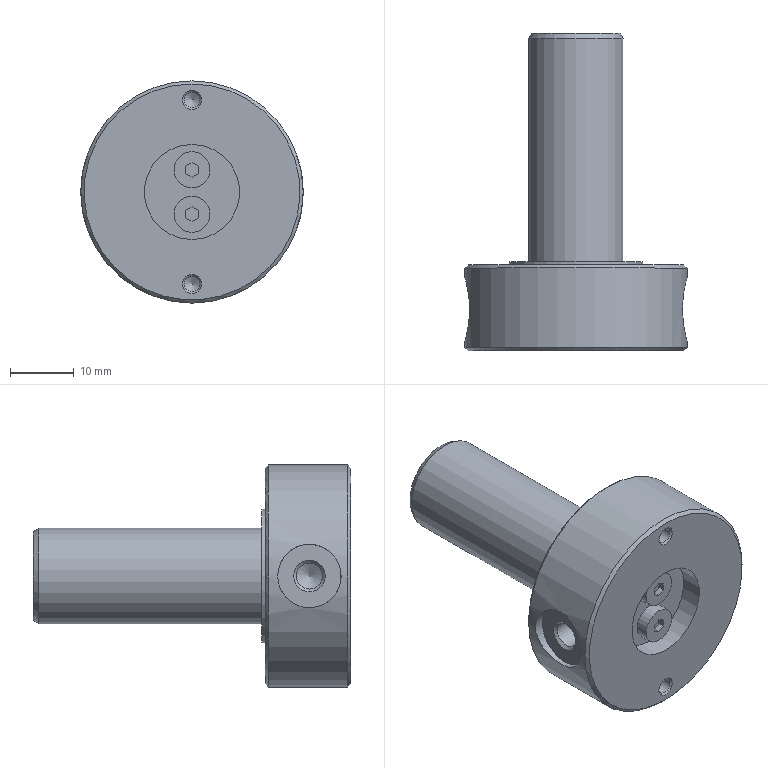Part | NX | 1 solid | 51 faces | box 35 x 50 x 35 mm | volume 18431 mm3 | plane 24 | cylinder 14 | cone 13 | commonest cylinder face diameters 2.459 x2 4.134 x2 5.7 x2 10 x2 15 x2 3 x1
STEP:
#1=CARTESIAN_POINT('',(0.,14.,-7.5));
#2=VERTEX_POINT('',#1);
#3=CARTESIAN_POINT('',(0.,14.,0.));
#4=DIRECTION('',(0.,-1.,0.));
#5=DIRECTION('',(0.,0.,-1.));
#6=AXIS2_PLACEMENT_3D('',#3,#4,#5);
#7=CIRCLE('',#6,7.5);
#8=EDGE_CURVE('',#2,#2,#7,.F.);
#9=ORIENTED_EDGE('',*,*,#8,.T.);
#10=EDGE_LOOP('',(#9));
#11=FACE_BOUND('',#10,.T.);
#12=CARTESIAN_POINT('',(0.,49.13,-7.5));
#13=VERTEX_POINT('',#12);
#14=CARTESIAN_POINT('',(0.,49.13,0.));
#15=DIRECTION('',(0.,-1.,0.));
#16=DIRECTION('',(0.,0.,-1.));
#17=AXIS2_PLACEMENT_3D('',#14,#15,#16);
#18=CIRCLE('',#17,7.5);
#19=EDGE_CURVE('',#13,#13,#18,.T.);
#20=ORIENTED_EDGE('',*,*,#19,.T.);
#21=EDGE_LOOP('',(#20));
#22=FACE_BOUND('',#21,.T.);
#23=CARTESIAN_POINT('',(0.,31.565,0.));
#24=DIRECTION('',(0.,-1.,0.));
#25=DIRECTION('',(0.,0.,-1.));
#26=AXIS2_PLACEMENT_3D('',#23,#24,#25);
#27=CYLINDRICAL_SURFACE('',#26,7.5);
#28=ADVANCED_FACE('',(#11,#22),#27,.T.);
#29=CARTESIAN_POINT('',(0.,50.,-7.));
#30=VERTEX_POINT('',#29);
#31=CARTESIAN_POINT('',(0.,50.,0.));
#32=DIRECTION('',(0.,-1.,0.));
#33=DIRECTION('',(0.,0.,-1.));
#34=AXIS2_PLACEMENT_3D('',#31,#32,#33);
#35=CIRCLE('',#34,7.);
#36=EDGE_CURVE('',#30,#30,#35,.T.);
#37=ORIENTED_EDGE('',*,*,#36,.T.);
#38=EDGE_LOOP('',(#37));
#39=FACE_BOUND('',#38,.T.);
#40=ORIENTED_EDGE('',*,*,#19,.F.);
#41=EDGE_LOOP('',(#40));
#42=FACE_BOUND('',#41,.T.);
#43=CARTESIAN_POINT('',(0.,49.13,0.));
#44=DIRECTION('',(0.,-1.,0.));
#45=DIRECTION('',(0.,0.,-1.));
#46=AXIS2_PLACEMENT_3D('',#43,#44,#45);
#47=CONICAL_SURFACE('',#46,7.5,0.5216);
#48=ADVANCED_FACE('',(#39,#42),#47,.T.);
#49=CARTESIAN_POINT('',(0.,14.,-10.5));
#50=VERTEX_POINT('',#49);
#51=CARTESIAN_POINT('',(0.,14.,0.));
#52=DIRECTION('',(0.,-1.,0.));
#53=DIRECTION('',(0.,0.,-1.));
#54=AXIS2_PLACEMENT_3D('',#51,#52,#53);
#55=CIRCLE('',#54,10.5);
#56=EDGE_CURVE('',#50,#50,#55,.F.);
#57=ORIENTED_EDGE('',*,*,#56,.T.);
#58=EDGE_LOOP('',(#57));
#59=FACE_BOUND('',#58,.T.);
#60=ORIENTED_EDGE('',*,*,#8,.F.);
#61=EDGE_LOOP('',(#60));
#62=FACE_BOUND('',#61,.T.);
#63=CARTESIAN_POINT('',(9.,14.,0.));
#64=DIRECTION('',(0.,1.,0.));
#65=DIRECTION('',(0.,0.,1.));
#66=AXIS2_PLACEMENT_3D('',#63,#64,#65);
#67=PLANE('',#66);
#68=ADVANCED_FACE('',(#59,#62),#67,.T.);
#69=ORIENTED_EDGE('',*,*,#36,.F.);
#70=EDGE_LOOP('',(#69));
#71=FACE_BOUND('',#70,.T.);
#72=CARTESIAN_POINT('',(0.,50.,2.));
#73=VERTEX_POINT('',#72);
#74=CARTESIAN_POINT('',(0.,50.,0.));
#75=DIRECTION('',(0.,1.,0.));
#76=DIRECTION('',(0.,0.,1.));
#77=AXIS2_PLACEMENT_3D('',#74,#75,#76);
#78=CIRCLE('',#77,2.);
#79=EDGE_CURVE('',#73,#73,#78,.F.);
#80=ORIENTED_EDGE('',*,*,#79,.T.);
#81=EDGE_LOOP('',(#80));
#82=FACE_BOUND('',#81,.T.);
#83=CARTESIAN_POINT('',(0.,50.,-6.));
#84=VERTEX_POINT('',#83);
#85=CARTESIAN_POINT('',(0.,50.,-4.5));
#86=DIRECTION('',(0.,-1.,0.));
#87=DIRECTION('',(0.,0.,-1.));
#88=AXIS2_PLACEMENT_3D('',#85,#86,#87);
#89=CIRCLE('',#88,1.5);
#90=EDGE_CURVE('',#84,#84,#89,.T.);
#91=ORIENTED_EDGE('',*,*,#90,.T.);
#92=EDGE_LOOP('',(#91));
#93=FACE_BOUND('',#92,.T.);
#94=CARTESIAN_POINT('',(3.5,50.,0.));
#95=DIRECTION('',(0.,1.,0.));
#96=DIRECTION('',(0.,0.,1.));
#97=AXIS2_PLACEMENT_3D('',#94,#95,#96);
#98=PLANE('',#97);
#99=ADVANCED_FACE('',(#71,#82,#93),#98,.T.);
#100=ORIENTED_EDGE('',*,*,#56,.F.);
#101=EDGE_LOOP('',(#100));
#102=FACE_BOUND('',#101,.T.);
#103=CARTESIAN_POINT('',(0.,13.5,-10.5));
#104=VERTEX_POINT('',#103);
#105=CARTESIAN_POINT('',(0.,13.5,0.));
#106=DIRECTION('',(0.,-1.,0.));
#107=DIRECTION('',(0.,0.,-1.));
#108=AXIS2_PLACEMENT_3D('',#105,#106,#107);
#109=CIRCLE('',#108,10.5);
#110=EDGE_CURVE('',#104,#104,#109,.F.);
#111=ORIENTED_EDGE('',*,*,#110,.T.);
#112=EDGE_LOOP('',(#111));
#113=FACE_BOUND('',#112,.T.);
#114=CARTESIAN_POINT('',(0.,13.75,0.));
#115=DIRECTION('',(0.,-1.,0.));
#116=DIRECTION('',(0.,0.,-1.));
#117=AXIS2_PLACEMENT_3D('',#114,#115,#116);
#118=CYLINDRICAL_SURFACE('',#117,10.5);
#119=ADVANCED_FACE('',(#102,#113),#118,.T.);
#120=ORIENTED_EDGE('',*,*,#79,.F.);
#121=EDGE_LOOP('',(#120));
#122=FACE_BOUND('',#121,.T.);
#123=CARTESIAN_POINT('',(1.621,49.621,0.));
#124=VERTEX_POINT('',#123);
#125=CARTESIAN_POINT('',(0.,49.621,0.));
#126=DIRECTION('',(0.,1.,0.));
#127=DIRECTION('',(1.,0.,0.));
#128=AXIS2_PLACEMENT_3D('',#125,#126,#127);
#129=CIRCLE('',#128,1.621);
#130=EDGE_CURVE('',#124,#124,#129,.T.);
#131=ORIENTED_EDGE('',*,*,#130,.F.);
#132=EDGE_LOOP('',(#131));
#133=FACE_BOUND('',#132,.T.);
#134=CARTESIAN_POINT('',(0.,50.,0.));
#135=DIRECTION('',(0.,1.,0.));
#136=DIRECTION('',(0.,0.,1.));
#137=AXIS2_PLACEMENT_3D('',#134,#135,#136);
#138=CONICAL_SURFACE('',#137,2.,0.7854);
#139=ADVANCED_FACE('',(#122,#133),#138,.F.);
#140=ORIENTED_EDGE('',*,*,#90,.F.);
#141=EDGE_LOOP('',(#140));
#142=FACE_BOUND('',#141,.T.);
#143=CARTESIAN_POINT('',(0.,40.,-6.));
#144=VERTEX_POINT('',#143);
#145=CARTESIAN_POINT('',(0.,40.,-4.5));
#146=DIRECTION('',(0.,-1.,0.));
#147=DIRECTION('',(0.,0.,-1.));
#148=AXIS2_PLACEMENT_3D('',#145,#146,#147);
#149=CIRCLE('',#148,1.5);
#150=EDGE_CURVE('',#144,#144,#149,.F.);
#151=ORIENTED_EDGE('',*,*,#150,.F.);
#152=EDGE_LOOP('',(#151));
#153=FACE_BOUND('',#152,.T.);
#154=CARTESIAN_POINT('',(0.,45.,-4.5));
#155=DIRECTION('',(0.,-1.,0.));
#156=DIRECTION('',(0.,0.,-1.));
#157=AXIS2_PLACEMENT_3D('',#154,#155,#156);
#158=CYLINDRICAL_SURFACE('',#157,1.5);
#159=ADVANCED_FACE('',(#142,#153),#158,.F.);
#160=CARTESIAN_POINT('',(0.,13.5,-17.));
#161=VERTEX_POINT('',#160);
#162=CARTESIAN_POINT('',(0.,13.5,0.));
#163=DIRECTION('',(0.,-1.,0.));
#164=DIRECTION('',(0.,0.,-1.));
#165=AXIS2_PLACEMENT_3D('',#162,#163,#164);
#166=CIRCLE('',#165,17.);
#167=EDGE_CURVE('',#161,#161,#166,.F.);
#168=ORIENTED_EDGE('',*,*,#167,.T.);
#169=EDGE_LOOP('',(#168));
#170=FACE_BOUND('',#169,.T.);
#171=ORIENTED_EDGE('',*,*,#110,.F.);
#172=EDGE_LOOP('',(#171));
#173=FACE_BOUND('',#172,.T.);
#174=CARTESIAN_POINT('',(13.75,13.5,0.));
#175=DIRECTION('',(0.,1.,0.));
#176=DIRECTION('',(0.,0.,1.));
#177=AXIS2_PLACEMENT_3D('',#174,#175,#176);
#178=PLANE('',#177);
#179=ADVANCED_FACE('',(#170,#173),#178,.T.);
#180=ORIENTED_EDGE('',*,*,#130,.T.);
#181=EDGE_LOOP('',(#180));
#182=FACE_BOUND('',#181,.T.);
#183=CARTESIAN_POINT('',(0.,42.,-1.621));
#184=VERTEX_POINT('',#183);
#185=CARTESIAN_POINT('',(0.,42.,0.));
#186=DIRECTION('',(0.,-1.,0.));
#187=DIRECTION('',(0.,0.,-1.));
#188=AXIS2_PLACEMENT_3D('',#185,#186,#187);
#189=CIRCLE('',#188,1.621);
#190=EDGE_CURVE('',#184,#184,#189,.F.);
#191=ORIENTED_EDGE('',*,*,#190,.F.);
#192=EDGE_LOOP('',(#191));
#193=FACE_BOUND('',#192,.T.);
#194=CARTESIAN_POINT('',(0.,45.81,0.));
#195=DIRECTION('',(0.,-1.,0.));
#196=DIRECTION('',(0.,0.,-1.));
#197=AXIS2_PLACEMENT_3D('',#194,#195,#196);
#198=CYLINDRICAL_SURFACE('',#197,1.621);
#199=ADVANCED_FACE('',(#182,#193),#198,.F.);
#200=ORIENTED_EDGE('',*,*,#150,.T.);
#201=EDGE_LOOP('',(#200));
#202=FACE_BOUND('',#201,.T.);
#203=CARTESIAN_POINT('',(0.,40.,-5.25));
#204=DIRECTION('',(0.,-1.,0.));
#205=DIRECTION('',(0.,0.,-1.));
#206=AXIS2_PLACEMENT_3D('',#203,#204,#205);
#207=PLANE('',#206);
#208=ADVANCED_FACE('',(#202),#207,.F.);
#209=ORIENTED_EDGE('',*,*,#167,.F.);
#210=EDGE_LOOP('',(#209));
#211=FACE_BOUND('',#210,.T.);
#212=CARTESIAN_POINT('',(17.5,13.,0.));
#213=VERTEX_POINT('',#212);
#214=CARTESIAN_POINT('',(0.,13.,0.));
#215=DIRECTION('',(0.,-1.,0.));
#216=DIRECTION('',(1.,0.,0.));
#217=AXIS2_PLACEMENT_3D('',#214,#215,#216);
#218=CIRCLE('',#217,17.5);
#219=EDGE_CURVE('',#213,#213,#218,.F.);
#220=ORIENTED_EDGE('',*,*,#219,.T.);
#221=EDGE_LOOP('',(#220));
#222=FACE_BOUND('',#221,.T.);
#223=CARTESIAN_POINT('',(0.,13.,0.));
#224=DIRECTION('',(0.,-1.,0.));
#225=DIRECTION('',(0.,0.,-1.));
#226=AXIS2_PLACEMENT_3D('',#223,#224,#225);
#227=CONICAL_SURFACE('',#226,17.5,0.7854);
#228=ADVANCED_FACE('',(#211,#222),#227,.T.);
#229=CARTESIAN_POINT('',(0.,41.064,0.));
#230=VERTEX_POINT('',#229);
#231=VERTEX_LOOP('',#230);
#232=FACE_BOUND('',#231,.T.);
#233=ORIENTED_EDGE('',*,*,#190,.T.);
#234=EDGE_LOOP('',(#233));
#235=FACE_BOUND('',#234,.T.);
#236=CARTESIAN_POINT('',(0.,42.,0.));
#237=DIRECTION('',(0.,1.,0.));
#238=DIRECTION('',(0.,0.,1.));
#239=AXIS2_PLACEMENT_3D('',#236,#237,#238);
#240=CONICAL_SURFACE('',#239,1.621,1.047);
#241=ADVANCED_FACE('',(#232,#235),#240,.F.);
#242=CARTESIAN_POINT('',(17.5,1.5,0.));
#243=VERTEX_POINT('',#242);
#244=CARTESIAN_POINT('',(17.143,2.584,-3.92));
#245=CARTESIAN_POINT('',(17.679,0.9588,0.0006164));
#246=CARTESIAN_POINT('',(17.143,2.581,3.917));
#247=CARTESIAN_POINT('',(16.584,6.501,5.541));
#248=CARTESIAN_POINT('',(17.143,10.416,3.92));
#249=CARTESIAN_POINT('',(17.679,12.041,-0.00121));
#250=CARTESIAN_POINT('',(17.143,10.419,-3.917));
#251=CARTESIAN_POINT('',(16.584,6.499,-5.541));
#252=CARTESIAN_POINT('',(17.143,2.584,-3.92));
#253=CARTESIAN_POINT('',(17.679,0.9588,0.0006164));
#254=CARTESIAN_POINT('',(17.143,2.581,3.917));
#255=B_SPLINE_CURVE_WITH_KNOTS('',3,(#244,#245,#246,#247,#248,#249,#250,#251,#252,#253,#254),.UNSPECIFIED.,.T.,.F.,(1,1,1,1,1,1,1,1,1,1,1,1,1,1,1),(-0.01963,-0.0157,-0.01178,-0.007852,-0.003926,0.000000332,0.003926,0.007852,0.01178,0.0157,0.01963,0.02356,0.02748,0.03141,0.03533),.UNSPECIFIED.);
#256=EDGE_CURVE('',#243,#243,#255,.T.);
#257=ORIENTED_EDGE('',*,*,#256,.T.);
#258=EDGE_LOOP('',(#257));
#259=FACE_BOUND('',#258,.T.);
#260=ORIENTED_EDGE('',*,*,#219,.F.);
#261=EDGE_LOOP('',(#260));
#262=FACE_BOUND('',#261,.T.);
#263=CARTESIAN_POINT('',(-17.5,11.5,0.));
#264=VERTEX_POINT('',#263);
#265=CARTESIAN_POINT('',(-17.143,10.416,-3.92));
#266=CARTESIAN_POINT('',(-17.679,12.041,0.0006164));
#267=CARTESIAN_POINT('',(-17.143,10.419,3.917));
#268=CARTESIAN_POINT('',(-16.584,6.499,5.541));
#269=CARTESIAN_POINT('',(-17.143,2.584,3.92));
#270=CARTESIAN_POINT('',(-17.679,0.9588,-0.00121));
#271=CARTESIAN_POINT('',(-17.143,2.581,-3.917));
#272=CARTESIAN_POINT('',(-16.584,6.501,-5.541));
#273=CARTESIAN_POINT('',(-17.143,10.416,-3.92));
#274=CARTESIAN_POINT('',(-17.679,12.041,0.0006164));
#275=CARTESIAN_POINT('',(-17.143,10.419,3.917));
#276=B_SPLINE_CURVE_WITH_KNOTS('',3,(#265,#266,#267,#268,#269,#270,#271,#272,#273,#274,#275),.UNSPECIFIED.,.T.,.F.,(1,1,1,1,1,1,1,1,1,1,1,1,1,1,1),(-0.01963,-0.0157,-0.01178,-0.007852,-0.003926,0.000000332,0.003926,0.007852,0.01178,0.0157,0.01963,0.02356,0.02748,0.03141,0.03533),.UNSPECIFIED.);
#277=EDGE_CURVE('',#264,#264,#276,.T.);
#278=ORIENTED_EDGE('',*,*,#277,.T.);
#279=EDGE_LOOP('',(#278));
#280=FACE_BOUND('',#279,.T.);
#281=CARTESIAN_POINT('',(0.,0.5,-17.5));
#282=VERTEX_POINT('',#281);
#283=CARTESIAN_POINT('',(0.,0.5,0.));
#284=DIRECTION('',(0.,-1.,0.));
#285=DIRECTION('',(0.,0.,-1.));
#286=AXIS2_PLACEMENT_3D('',#283,#284,#285);
#287=CIRCLE('',#286,17.5);
#288=EDGE_CURVE('',#282,#282,#287,.F.);
#289=ORIENTED_EDGE('',*,*,#288,.T.);
#290=EDGE_LOOP('',(#289));
#291=FACE_BOUND('',#290,.T.);
#292=CARTESIAN_POINT('',(0.,6.75,0.));
#293=DIRECTION('',(0.,-1.,0.));
#294=DIRECTION('',(0.,0.,-1.));
#295=AXIS2_PLACEMENT_3D('',#292,#293,#294);
#296=CYLINDRICAL_SURFACE('',#295,17.5);
#297=ADVANCED_FACE('',(#259,#262,#280,#291),#296,.T.);
#298=ORIENTED_EDGE('',*,*,#288,.F.);
#299=EDGE_LOOP('',(#298));
#300=FACE_BOUND('',#299,.T.);
#301=CARTESIAN_POINT('',(0.,0.,17.));
#302=VERTEX_POINT('',#301);
#303=CARTESIAN_POINT('',(0.,0.,0.));
#304=DIRECTION('',(0.,1.,0.));
#305=DIRECTION('',(0.,0.,1.));
#306=AXIS2_PLACEMENT_3D('',#303,#304,#305);
#307=CIRCLE('',#306,17.);
#308=EDGE_CURVE('',#302,#302,#307,.T.);
#309=ORIENTED_EDGE('',*,*,#308,.T.);
#310=EDGE_LOOP('',(#309));
#311=FACE_BOUND('',#310,.T.);
#312=CARTESIAN_POINT('',(0.,0.5,0.));
#313=DIRECTION('',(0.,1.,0.));
#314=DIRECTION('',(0.,0.,1.));
#315=AXIS2_PLACEMENT_3D('',#312,#313,#314);
#316=CONICAL_SURFACE('',#315,17.5,0.7854);
#317=ADVANCED_FACE('',(#300,#311),#316,.T.);
#318=CARTESIAN_POINT('',(-16.,6.5,5.));
#319=VERTEX_POINT('',#318);
#320=CARTESIAN_POINT('',(-16.,6.5,0.));
#321=DIRECTION('',(-1.,0.,0.));
#322=DIRECTION('',(0.,0.,1.));
#323=AXIS2_PLACEMENT_3D('',#320,#321,#322);
#324=CIRCLE('',#323,5.);
#325=EDGE_CURVE('',#319,#319,#324,.T.);
#326=ORIENTED_EDGE('',*,*,#325,.F.);
#327=EDGE_LOOP('',(#326));
#328=FACE_BOUND('',#327,.T.);
#329=ORIENTED_EDGE('',*,*,#277,.F.);
#330=EDGE_LOOP('',(#329));
#331=FACE_BOUND('',#330,.T.);
#332=CARTESIAN_POINT('',(-16.75,6.5,0.));
#333=DIRECTION('',(-1.,0.,0.));
#334=DIRECTION('',(0.,0.,1.));
#335=AXIS2_PLACEMENT_3D('',#332,#333,#334);
#336=CYLINDRICAL_SURFACE('',#335,5.);
#337=ADVANCED_FACE('',(#328,#331),#336,.F.);
#338=ORIENTED_EDGE('',*,*,#256,.F.);
#339=EDGE_LOOP('',(#338));
#340=FACE_BOUND('',#339,.T.);
#341=CARTESIAN_POINT('',(16.,6.5,-5.));
#342=VERTEX_POINT('',#341);
#343=CARTESIAN_POINT('',(16.,6.5,0.));
#344=DIRECTION('',(1.,0.,0.));
#345=DIRECTION('',(0.,0.,-1.));
#346=AXIS2_PLACEMENT_3D('',#343,#344,#345);
#347=CIRCLE('',#346,5.);
#348=EDGE_CURVE('',#342,#342,#347,.T.);
#349=ORIENTED_EDGE('',*,*,#348,.F.);
#350=EDGE_LOOP('',(#349));
#351=FACE_BOUND('',#350,.T.);
#352=CARTESIAN_POINT('',(16.75,6.5,0.));
#353=DIRECTION('',(1.,0.,0.));
#354=DIRECTION('',(0.,0.,-1.));
#355=AXIS2_PLACEMENT_3D('',#352,#353,#354);
#356=CYLINDRICAL_SURFACE('',#355,5.);
#357=ADVANCED_FACE('',(#340,#351),#356,.F.);
#358=CARTESIAN_POINT('',(0.,0.,-7.5));
#359=VERTEX_POINT('',#358);
#360=CARTESIAN_POINT('',(0.,0.,0.));
#361=DIRECTION('',(0.,-1.,0.));
#362=DIRECTION('',(0.,0.,-1.));
#363=AXIS2_PLACEMENT_3D('',#360,#361,#362);
#364=CIRCLE('',#363,7.5);
#365=EDGE_CURVE('',#359,#359,#364,.F.);
#366=ORIENTED_EDGE('',*,*,#365,.T.);
#367=EDGE_LOOP('',(#366));
#368=FACE_BOUND('',#367,.T.);
#369=ORIENTED_EDGE('',*,*,#308,.F.);
#370=EDGE_LOOP('',(#369));
#371=FACE_BOUND('',#370,.T.);
#372=CARTESIAN_POINT('',(0.,0.,13.));
#373=VERTEX_POINT('',#372);
#374=CARTESIAN_POINT('',(0.,0.,14.5));
#375=DIRECTION('',(0.,-1.,0.));
#376=DIRECTION('',(0.,0.,-1.));
#377=AXIS2_PLACEMENT_3D('',#374,#375,#376);
#378=CIRCLE('',#377,1.5);
#379=EDGE_CURVE('',#373,#373,#378,.F.);
#380=ORIENTED_EDGE('',*,*,#379,.T.);
#381=EDGE_LOOP('',(#380));
#382=FACE_BOUND('',#381,.T.);
#383=CARTESIAN_POINT('',(0.,0.,-16.));
#384=VERTEX_POINT('',#383);
#385=CARTESIAN_POINT('',(0.,0.,-14.5));
#386=DIRECTION('',(0.,-1.,0.));
#387=DIRECTION('',(0.,0.,-1.));
#388=AXIS2_PLACEMENT_3D('',#385,#386,#387);
#389=CIRCLE('',#388,1.5);
#390=EDGE_CURVE('',#384,#384,#389,.F.);
#391=ORIENTED_EDGE('',*,*,#390,.T.);
#392=EDGE_LOOP('',(#391));
#393=FACE_BOUND('',#392,.T.);
#394=CARTESIAN_POINT('',(12.25,0.,0.));
#395=DIRECTION('',(0.,-1.,0.));
#396=DIRECTION('',(0.,0.,-1.));
#397=AXIS2_PLACEMENT_3D('',#394,#395,#396);
#398=PLANE('',#397);
#399=ADVANCED_FACE('',(#368,#371,#382,#393),#398,.T.);
#400=ORIENTED_EDGE('',*,*,#325,.T.);
#401=EDGE_LOOP('',(#400));
#402=FACE_BOUND('',#401,.T.);
#403=CARTESIAN_POINT('',(-16.,6.5,2.5));
#404=VERTEX_POINT('',#403);
#405=CARTESIAN_POINT('',(-16.,6.5,0.));
#406=DIRECTION('',(-1.,0.,0.));
#407=DIRECTION('',(0.,0.,1.));
#408=AXIS2_PLACEMENT_3D('',#405,#406,#407);
#409=CIRCLE('',#408,2.5);
#410=EDGE_CURVE('',#404,#404,#409,.T.);
#411=ORIENTED_EDGE('',*,*,#410,.F.);
#412=EDGE_LOOP('',(#411));
#413=FACE_BOUND('',#412,.T.);
#414=CARTESIAN_POINT('',(-16.,6.5,3.75));
#415=DIRECTION('',(1.,0.,0.));
#416=DIRECTION('',(0.,0.,-1.));
#417=AXIS2_PLACEMENT_3D('',#414,#415,#416);
#418=PLANE('',#417);
#419=ADVANCED_FACE('',(#402,#413),#418,.F.);
#420=ORIENTED_EDGE('',*,*,#348,.T.);
#421=EDGE_LOOP('',(#420));
#422=FACE_BOUND('',#421,.T.);
#423=CARTESIAN_POINT('',(16.,6.5,-2.5));
#424=VERTEX_POINT('',#423);
#425=CARTESIAN_POINT('',(16.,6.5,0.));
#426=DIRECTION('',(1.,0.,0.));
#427=DIRECTION('',(0.,0.,-1.));
#428=AXIS2_PLACEMENT_3D('',#425,#426,#427);
#429=CIRCLE('',#428,2.5);
#430=EDGE_CURVE('',#424,#424,#429,.T.);
#431=ORIENTED_EDGE('',*,*,#430,.F.);
#432=EDGE_LOOP('',(#431));
#433=FACE_BOUND('',#432,.T.);
#434=CARTESIAN_POINT('',(16.,6.5,-3.75));
#435=DIRECTION('',(-1.,0.,0.));
#436=DIRECTION('',(0.,0.,1.));
#437=AXIS2_PLACEMENT_3D('',#434,#435,#436);
#438=PLANE('',#437);
#439=ADVANCED_FACE('',(#422,#433),#438,.F.);
#440=ORIENTED_EDGE('',*,*,#365,.F.);
#441=EDGE_LOOP('',(#440));
#442=FACE_BOUND('',#441,.T.);
#443=CARTESIAN_POINT('',(0.,3.5,-7.5));
#444=VERTEX_POINT('',#443);
#445=CARTESIAN_POINT('',(0.,3.5,0.));
#446=DIRECTION('',(0.,-1.,0.));
#447=DIRECTION('',(0.,0.,-1.));
#448=AXIS2_PLACEMENT_3D('',#445,#446,#447);
#449=CIRCLE('',#448,7.5);
#450=EDGE_CURVE('',#444,#444,#449,.T.);
#451=ORIENTED_EDGE('',*,*,#450,.F.);
#452=EDGE_LOOP('',(#451));
#453=FACE_BOUND('',#452,.T.);
#454=CARTESIAN_POINT('',(0.,1.75,0.));
#455=DIRECTION('',(0.,-1.,0.));
#456=DIRECTION('',(0.,0.,-1.));
#457=AXIS2_PLACEMENT_3D('',#454,#455,#456);
#458=CYLINDRICAL_SURFACE('',#457,7.5);
#459=ADVANCED_FACE('',(#442,#453),#458,.F.);
#460=ORIENTED_EDGE('',*,*,#379,.F.);
#461=EDGE_LOOP('',(#460));
#462=FACE_BOUND('',#461,.T.);
#463=CARTESIAN_POINT('',(0.,0.2705,13.27));
#464=VERTEX_POINT('',#463);
#465=CARTESIAN_POINT('',(0.,0.2705,14.5));
#466=DIRECTION('',(0.,-1.,0.));
#467=DIRECTION('',(0.,0.,-1.));
#468=AXIS2_PLACEMENT_3D('',#465,#466,#467);
#469=CIRCLE('',#468,1.23);
#470=EDGE_CURVE('',#464,#464,#469,.T.);
#471=ORIENTED_EDGE('',*,*,#470,.F.);
#472=EDGE_LOOP('',(#471));
#473=FACE_BOUND('',#472,.T.);
#474=CARTESIAN_POINT('',(0.,0.,14.5));
#475=DIRECTION('',(0.,-1.,0.));
#476=DIRECTION('',(0.,0.,-1.));
#477=AXIS2_PLACEMENT_3D('',#474,#475,#476);
#478=CONICAL_SURFACE('',#477,1.5,0.7854);
#479=ADVANCED_FACE('',(#462,#473),#478,.F.);
#480=ORIENTED_EDGE('',*,*,#390,.F.);
#481=EDGE_LOOP('',(#480));
#482=FACE_BOUND('',#481,.T.);
#483=CARTESIAN_POINT('',(0.,0.2705,-15.729));
#484=VERTEX_POINT('',#483);
#485=CARTESIAN_POINT('',(0.,0.2705,-14.5));
#486=DIRECTION('',(0.,-1.,0.));
#487=DIRECTION('',(0.,0.,-1.));
#488=AXIS2_PLACEMENT_3D('',#485,#486,#487);
#489=CIRCLE('',#488,1.229);
#490=EDGE_CURVE('',#484,#484,#489,.T.);
#491=ORIENTED_EDGE('',*,*,#490,.F.);
#492=EDGE_LOOP('',(#491));
#493=FACE_BOUND('',#492,.T.);
#494=CARTESIAN_POINT('',(0.,0.,-14.5));
#495=DIRECTION('',(0.,-1.,0.));
#496=DIRECTION('',(0.,0.,-1.));
#497=AXIS2_PLACEMENT_3D('',#494,#495,#496);
#498=CONICAL_SURFACE('',#497,1.5,0.7854);
#499=ADVANCED_FACE('',(#482,#493),#498,.F.);
#500=CARTESIAN_POINT('',(-15.567,6.5,2.067));
#501=VERTEX_POINT('',#500);
#502=CARTESIAN_POINT('',(-15.567,6.5,0.));
#503=DIRECTION('',(-1.,0.,0.));
#504=DIRECTION('',(0.,0.,1.));
#505=AXIS2_PLACEMENT_3D('',#502,#503,#504);
#506=CIRCLE('',#505,2.067);
#507=EDGE_CURVE('',#501,#501,#506,.T.);
#508=ORIENTED_EDGE('',*,*,#507,.F.);
#509=EDGE_LOOP('',(#508));
#510=FACE_BOUND('',#509,.T.);
#511=ORIENTED_EDGE('',*,*,#410,.T.);
#512=EDGE_LOOP('',(#511));
#513=FACE_BOUND('',#512,.T.);
#514=CARTESIAN_POINT('',(-16.,6.5,0.));
#515=DIRECTION('',(-1.,0.,0.));
#516=DIRECTION('',(0.,0.,1.));
#517=AXIS2_PLACEMENT_3D('',#514,#515,#516);
#518=CONICAL_SURFACE('',#517,2.5,0.7854);
#519=ADVANCED_FACE('',(#510,#513),#518,.F.);
#520=CARTESIAN_POINT('',(15.567,6.5,-2.067));
#521=VERTEX_POINT('',#520);
#522=CARTESIAN_POINT('',(15.567,6.5,0.));
#523=DIRECTION('',(1.,0.,0.));
#524=DIRECTION('',(0.,0.,-1.));
#525=AXIS2_PLACEMENT_3D('',#522,#523,#524);
#526=CIRCLE('',#525,2.067);
#527=EDGE_CURVE('',#521,#521,#526,.T.);
#528=ORIENTED_EDGE('',*,*,#527,.F.);
#529=EDGE_LOOP('',(#528));
#530=FACE_BOUND('',#529,.T.);
#531=ORIENTED_EDGE('',*,*,#430,.T.);
#532=EDGE_LOOP('',(#531));
#533=FACE_BOUND('',#532,.T.);
#534=CARTESIAN_POINT('',(16.,6.5,0.));
#535=DIRECTION('',(1.,0.,0.));
#536=DIRECTION('',(0.,0.,-1.));
#537=AXIS2_PLACEMENT_3D('',#534,#535,#536);
#538=CONICAL_SURFACE('',#537,2.5,0.7854);
#539=ADVANCED_FACE('',(#530,#533),#538,.F.);
#540=ORIENTED_EDGE('',*,*,#450,.T.);
#541=EDGE_LOOP('',(#540));
#542=FACE_BOUND('',#541,.T.);
#543=CARTESIAN_POINT('',(0.,3.5,6.35));
#544=VERTEX_POINT('',#543);
#545=CARTESIAN_POINT('',(0.,3.5,3.5));
#546=DIRECTION('',(0.,1.,0.));
#547=DIRECTION('',(0.,0.,1.));
#548=AXIS2_PLACEMENT_3D('',#545,#546,#547);
#549=CIRCLE('',#548,2.85);
#550=EDGE_CURVE('',#544,#544,#549,.T.);
#551=ORIENTED_EDGE('',*,*,#550,.T.);
#552=EDGE_LOOP('',(#551));
#553=FACE_BOUND('',#552,.T.);
#554=CARTESIAN_POINT('',(0.,3.5,-0.65));
#555=VERTEX_POINT('',#554);
#556=CARTESIAN_POINT('',(0.,3.5,-3.5));
#557=DIRECTION('',(0.,1.,0.));
#558=DIRECTION('',(0.,0.,1.));
#559=AXIS2_PLACEMENT_3D('',#556,#557,#558);
#560=CIRCLE('',#559,2.85);
#561=EDGE_CURVE('',#555,#555,#560,.T.);
#562=ORIENTED_EDGE('',*,*,#561,.T.);
#563=EDGE_LOOP('',(#562));
#564=FACE_BOUND('',#563,.T.);
#565=CARTESIAN_POINT('',(3.75,3.5,0.));
#566=DIRECTION('',(0.,-1.,0.));
#567=DIRECTION('',(0.,0.,-1.));
#568=AXIS2_PLACEMENT_3D('',#565,#566,#567);
#569=PLANE('',#568);
#570=ADVANCED_FACE('',(#542,#553,#564),#569,.T.);
#571=ORIENTED_EDGE('',*,*,#470,.T.);
#572=EDGE_LOOP('',(#571));
#573=FACE_BOUND('',#572,.T.);
#574=CARTESIAN_POINT('',(0.,8.,13.271));
#575=VERTEX_POINT('',#574);
#576=CARTESIAN_POINT('',(0.,8.,14.5));
#577=DIRECTION('',(0.,-1.,0.));
#578=DIRECTION('',(0.,0.,-1.));
#579=AXIS2_PLACEMENT_3D('',#576,#577,#578);
#580=CIRCLE('',#579,1.23);
#581=EDGE_CURVE('',#575,#575,#580,.T.);
#582=ORIENTED_EDGE('',*,*,#581,.F.);
#583=EDGE_LOOP('',(#582));
#584=FACE_BOUND('',#583,.T.);
#585=CARTESIAN_POINT('',(0.,4.135,14.5));
#586=DIRECTION('',(0.,-1.,0.));
#587=DIRECTION('',(0.,0.,-1.));
#588=AXIS2_PLACEMENT_3D('',#585,#586,#587);
#589=CYLINDRICAL_SURFACE('',#588,1.23);
#590=ADVANCED_FACE('',(#573,#584),#589,.F.);
#591=ORIENTED_EDGE('',*,*,#490,.T.);
#592=EDGE_LOOP('',(#591));
#593=FACE_BOUND('',#592,.T.);
#594=CARTESIAN_POINT('',(0.,8.,-15.729));
#595=VERTEX_POINT('',#594);
#596=CARTESIAN_POINT('',(0.,8.,-14.5));
#597=DIRECTION('',(0.,-1.,0.));
#598=DIRECTION('',(0.,0.,-1.));
#599=AXIS2_PLACEMENT_3D('',#596,#597,#598);
#600=CIRCLE('',#599,1.23);
#601=EDGE_CURVE('',#595,#595,#600,.T.);
#602=ORIENTED_EDGE('',*,*,#601,.F.);
#603=EDGE_LOOP('',(#602));
#604=FACE_BOUND('',#603,.T.);
#605=CARTESIAN_POINT('',(0.,4.135,-14.5));
#606=DIRECTION('',(0.,-1.,0.));
#607=DIRECTION('',(0.,0.,-1.));
#608=AXIS2_PLACEMENT_3D('',#605,#606,#607);
#609=CYLINDRICAL_SURFACE('',#608,1.23);
#610=ADVANCED_FACE('',(#593,#604),#609,.F.);
#611=CARTESIAN_POINT('',(-12.5,6.5,2.067));
#612=VERTEX_POINT('',#611);
#613=CARTESIAN_POINT('',(-12.5,6.5,0.));
#614=DIRECTION('',(-1.,0.,0.));
#615=DIRECTION('',(0.,0.,1.));
#616=AXIS2_PLACEMENT_3D('',#613,#614,#615);
#617=CIRCLE('',#616,2.067);
#618=EDGE_CURVE('',#612,#612,#617,.T.);
#619=ORIENTED_EDGE('',*,*,#618,.F.);
#620=EDGE_LOOP('',(#619));
#621=FACE_BOUND('',#620,.T.);
#622=ORIENTED_EDGE('',*,*,#507,.T.);
#623=EDGE_LOOP('',(#622));
#624=FACE_BOUND('',#623,.T.);
#625=CARTESIAN_POINT('',(-14.034,6.5,0.));
#626=DIRECTION('',(-1.,0.,0.));
#627=DIRECTION('',(0.,0.,1.));
#628=AXIS2_PLACEMENT_3D('',#625,#626,#627);
#629=CYLINDRICAL_SURFACE('',#628,2.067);
#630=ADVANCED_FACE('',(#621,#624),#629,.F.);
#631=CARTESIAN_POINT('',(12.5,6.5,-2.067));
#632=VERTEX_POINT('',#631);
#633=CARTESIAN_POINT('',(12.5,6.5,0.));
#634=DIRECTION('',(1.,0.,0.));
#635=DIRECTION('',(0.,0.,-1.));
#636=AXIS2_PLACEMENT_3D('',#633,#634,#635);
#637=CIRCLE('',#636,2.067);
#638=EDGE_CURVE('',#632,#632,#637,.T.);
#639=ORIENTED_EDGE('',*,*,#638,.F.);
#640=EDGE_LOOP('',(#639));
#641=FACE_BOUND('',#640,.T.);
#642=ORIENTED_EDGE('',*,*,#527,.T.);
#643=EDGE_LOOP('',(#642));
#644=FACE_BOUND('',#643,.T.);
#645=CARTESIAN_POINT('',(14.034,6.5,0.));
#646=DIRECTION('',(1.,0.,0.));
#647=DIRECTION('',(0.,0.,-1.));
#648=AXIS2_PLACEMENT_3D('',#645,#646,#647);
#649=CYLINDRICAL_SURFACE('',#648,2.067);
#650=ADVANCED_FACE('',(#641,#644),#649,.F.);
#651=ORIENTED_EDGE('',*,*,#550,.F.);
#652=EDGE_LOOP('',(#651));
#653=FACE_BOUND('',#652,.T.);
#654=CARTESIAN_POINT('',(0.,1.5,6.35));
#655=VERTEX_POINT('',#654);
#656=CARTESIAN_POINT('',(0.,1.5,3.5));
#657=DIRECTION('',(0.,1.,0.));
#658=DIRECTION('',(0.,0.,1.));
#659=AXIS2_PLACEMENT_3D('',#656,#657,#658);
#660=CIRCLE('',#659,2.85);
#661=EDGE_CURVE('',#655,#655,#660,.T.);
#662=ORIENTED_EDGE('',*,*,#661,.T.);
#663=EDGE_LOOP('',(#662));
#664=FACE_BOUND('',#663,.T.);
#665=CARTESIAN_POINT('',(0.,2.5,3.5));
#666=DIRECTION('',(0.,1.,0.));
#667=DIRECTION('',(0.,0.,1.));
#668=AXIS2_PLACEMENT_3D('',#665,#666,#667);
#669=CYLINDRICAL_SURFACE('',#668,2.85);
#670=ADVANCED_FACE('',(#653,#664),#669,.T.);
#671=ORIENTED_EDGE('',*,*,#561,.F.);
#672=EDGE_LOOP('',(#671));
#673=FACE_BOUND('',#672,.T.);
#674=CARTESIAN_POINT('',(0.,1.5,-0.65));
#675=VERTEX_POINT('',#674);
#676=CARTESIAN_POINT('',(0.,1.5,-3.5));
#677=DIRECTION('',(0.,1.,0.));
#678=DIRECTION('',(0.,0.,1.));
#679=AXIS2_PLACEMENT_3D('',#676,#677,#678);
#680=CIRCLE('',#679,2.85);
#681=EDGE_CURVE('',#675,#675,#680,.T.);
#682=ORIENTED_EDGE('',*,*,#681,.T.);
#683=EDGE_LOOP('',(#682));
#684=FACE_BOUND('',#683,.T.);
#685=CARTESIAN_POINT('',(0.,2.5,-3.5));
#686=DIRECTION('',(0.,1.,0.));
#687=DIRECTION('',(0.,0.,1.));
#688=AXIS2_PLACEMENT_3D('',#685,#686,#687);
#689=CYLINDRICAL_SURFACE('',#688,2.85);
#690=ADVANCED_FACE('',(#673,#684),#689,.T.);
#691=CARTESIAN_POINT('',(0.,8.71,14.5));
#692=VERTEX_POINT('',#691);
#693=VERTEX_LOOP('',#692);
#694=FACE_BOUND('',#693,.T.);
#695=ORIENTED_EDGE('',*,*,#581,.T.);
#696=EDGE_LOOP('',(#695));
#697=FACE_BOUND('',#696,.T.);
#698=CARTESIAN_POINT('',(0.,8.,14.5));
#699=DIRECTION('',(0.,-1.,0.));
#700=DIRECTION('',(0.,0.,-1.));
#701=AXIS2_PLACEMENT_3D('',#698,#699,#700);
#702=CONICAL_SURFACE('',#701,1.229,1.047);
#703=ADVANCED_FACE('',(#694,#697),#702,.F.);
#704=CARTESIAN_POINT('',(0.,8.71,-14.5));
#705=VERTEX_POINT('',#704);
#706=VERTEX_LOOP('',#705);
#707=FACE_BOUND('',#706,.T.);
#708=ORIENTED_EDGE('',*,*,#601,.T.);
#709=EDGE_LOOP('',(#708));
#710=FACE_BOUND('',#709,.T.);
#711=CARTESIAN_POINT('',(0.,8.,-14.5));
#712=DIRECTION('',(0.,-1.,0.));
#713=DIRECTION('',(0.,0.,-1.));
#714=AXIS2_PLACEMENT_3D('',#711,#712,#713);
#715=CONICAL_SURFACE('',#714,1.229,1.047);
#716=ADVANCED_FACE('',(#707,#710),#715,.F.);
#717=ORIENTED_EDGE('',*,*,#618,.T.);
#718=EDGE_LOOP('',(#717));
#719=FACE_BOUND('',#718,.T.);
#720=CARTESIAN_POINT('',(-11.307,6.5,0.));
#721=VERTEX_POINT('',#720);
#722=VERTEX_LOOP('',#721);
#723=FACE_BOUND('',#722,.T.);
#724=CARTESIAN_POINT('',(-12.5,6.5,0.));
#725=DIRECTION('',(-1.,0.,0.));
#726=DIRECTION('',(0.,0.,1.));
#727=AXIS2_PLACEMENT_3D('',#724,#725,#726);
#728=CONICAL_SURFACE('',#727,2.067,1.047);
#729=ADVANCED_FACE('',(#719,#723),#728,.F.);
#730=ORIENTED_EDGE('',*,*,#638,.T.);
#731=EDGE_LOOP('',(#730));
#732=FACE_BOUND('',#731,.T.);
#733=CARTESIAN_POINT('',(11.307,6.5,0.));
#734=VERTEX_POINT('',#733);
#735=VERTEX_LOOP('',#734);
#736=FACE_BOUND('',#735,.T.);
#737=CARTESIAN_POINT('',(12.5,6.5,0.));
#738=DIRECTION('',(1.,0.,0.));
#739=DIRECTION('',(0.,0.,-1.));
#740=AXIS2_PLACEMENT_3D('',#737,#738,#739);
#741=CONICAL_SURFACE('',#740,2.067,1.047);
#742=ADVANCED_FACE('',(#732,#736),#741,.F.);
#743=ORIENTED_EDGE('',*,*,#661,.F.);
#744=EDGE_LOOP('',(#743));
#745=FACE_BOUND('',#744,.T.);
#746=CARTESIAN_POINT('',(1.,1.5,4.077));
#747=VERTEX_POINT('',#746);
#748=CARTESIAN_POINT('',(1.,1.5,2.923));
#749=VERTEX_POINT('',#748);
#750=CARTESIAN_POINT('',(1.,1.5,4.925));
#751=DIRECTION('',(0.,0.,-1.));
#752=VECTOR('',#751,1000.);
#753=LINE('',#750,#752);
#754=EDGE_CURVE('',#747,#749,#753,.T.);
#755=ORIENTED_EDGE('',*,*,#754,.T.);
#756=CARTESIAN_POINT('',(0.,1.5,2.345));
#757=VERTEX_POINT('',#756);
#758=CARTESIAN_POINT('',(1.,1.5,2.923));
#759=DIRECTION('',(-0.866,0.,-0.5));
#760=VECTOR('',#759,1000.);
#761=LINE('',#758,#760);
#762=EDGE_CURVE('',#749,#757,#761,.T.);
#763=ORIENTED_EDGE('',*,*,#762,.T.);
#764=CARTESIAN_POINT('',(-1.,1.5,2.923));
#765=VERTEX_POINT('',#764);
#766=CARTESIAN_POINT('',(0.,1.5,2.345));
#767=DIRECTION('',(-0.866,0.,0.5));
#768=VECTOR('',#767,1000.);
#769=LINE('',#766,#768);
#770=EDGE_CURVE('',#757,#765,#769,.T.);
#771=ORIENTED_EDGE('',*,*,#770,.T.);
#772=CARTESIAN_POINT('',(-1.,1.5,4.077));
#773=VERTEX_POINT('',#772);
#774=CARTESIAN_POINT('',(-1.,1.5,4.925));
#775=DIRECTION('',(0.,0.,-1.));
#776=VECTOR('',#775,1000.);
#777=LINE('',#774,#776);
#778=EDGE_CURVE('',#765,#773,#777,.F.);
#779=ORIENTED_EDGE('',*,*,#778,.T.);
#780=CARTESIAN_POINT('',(0.,1.5,4.655));
#781=VERTEX_POINT('',#780);
#782=CARTESIAN_POINT('',(-1.,1.5,4.077));
#783=DIRECTION('',(0.866,0.,0.5));
#784=VECTOR('',#783,1000.);
#785=LINE('',#782,#784);
#786=EDGE_CURVE('',#773,#781,#785,.T.);
#787=ORIENTED_EDGE('',*,*,#786,.T.);
#788=CARTESIAN_POINT('',(0.,1.5,4.655));
#789=DIRECTION('',(0.866,0.,-0.5));
#790=VECTOR('',#789,1000.);
#791=LINE('',#788,#790);
#792=EDGE_CURVE('',#781,#747,#791,.T.);
#793=ORIENTED_EDGE('',*,*,#792,.T.);
#794=EDGE_LOOP('',(#755,#763,#771,#779,#787,#793));
#795=FACE_BOUND('',#794,.T.);
#796=CARTESIAN_POINT('',(0.,1.5,4.925));
#797=DIRECTION('',(0.,-1.,0.));
#798=DIRECTION('',(0.,0.,-1.));
#799=AXIS2_PLACEMENT_3D('',#796,#797,#798);
#800=PLANE('',#799);
#801=ADVANCED_FACE('',(#745,#795),#800,.T.);
#802=ORIENTED_EDGE('',*,*,#681,.F.);
#803=EDGE_LOOP('',(#802));
#804=FACE_BOUND('',#803,.T.);
#805=CARTESIAN_POINT('',(1.,1.5,-2.923));
#806=VERTEX_POINT('',#805);
#807=CARTESIAN_POINT('',(1.,1.5,-4.077));
#808=VERTEX_POINT('',#807);
#809=CARTESIAN_POINT('',(1.,1.5,-2.075));
#810=DIRECTION('',(0.,0.,-1.));
#811=VECTOR('',#810,1000.);
#812=LINE('',#809,#811);
#813=EDGE_CURVE('',#806,#808,#812,.T.);
#814=ORIENTED_EDGE('',*,*,#813,.T.);
#815=CARTESIAN_POINT('',(0.,1.5,-4.655));
#816=VERTEX_POINT('',#815);
#817=CARTESIAN_POINT('',(1.,1.5,-4.077));
#818=DIRECTION('',(-0.866,0.,-0.5));
#819=VECTOR('',#818,1000.);
#820=LINE('',#817,#819);
#821=EDGE_CURVE('',#808,#816,#820,.T.);
#822=ORIENTED_EDGE('',*,*,#821,.T.);
#823=CARTESIAN_POINT('',(-1.,1.5,-4.077));
#824=VERTEX_POINT('',#823);
#825=CARTESIAN_POINT('',(0.,1.5,-4.655));
#826=DIRECTION('',(-0.866,0.,0.5));
#827=VECTOR('',#826,1000.);
#828=LINE('',#825,#827);
#829=EDGE_CURVE('',#816,#824,#828,.T.);
#830=ORIENTED_EDGE('',*,*,#829,.T.);
#831=CARTESIAN_POINT('',(-1.,1.5,-2.923));
#832=VERTEX_POINT('',#831);
#833=CARTESIAN_POINT('',(-1.,1.5,-2.075));
#834=DIRECTION('',(0.,0.,-1.));
#835=VECTOR('',#834,1000.);
#836=LINE('',#833,#835);
#837=EDGE_CURVE('',#824,#832,#836,.F.);
#838=ORIENTED_EDGE('',*,*,#837,.T.);
#839=CARTESIAN_POINT('',(0.,1.5,-2.345));
#840=VERTEX_POINT('',#839);
#841=CARTESIAN_POINT('',(-1.,1.5,-2.923));
#842=DIRECTION('',(0.866,0.,0.5));
#843=VECTOR('',#842,1000.);
#844=LINE('',#841,#843);
#845=EDGE_CURVE('',#832,#840,#844,.T.);
#846=ORIENTED_EDGE('',*,*,#845,.T.);
#847=CARTESIAN_POINT('',(0.,1.5,-2.345));
#848=DIRECTION('',(0.866,0.,-0.5));
#849=VECTOR('',#848,1000.);
#850=LINE('',#847,#849);
#851=EDGE_CURVE('',#840,#806,#850,.T.);
#852=ORIENTED_EDGE('',*,*,#851,.T.);
#853=EDGE_LOOP('',(#814,#822,#830,#838,#846,#852));
#854=FACE_BOUND('',#853,.T.);
#855=CARTESIAN_POINT('',(0.,1.5,-2.075));
#856=DIRECTION('',(0.,-1.,0.));
#857=DIRECTION('',(0.,0.,-1.));
#858=AXIS2_PLACEMENT_3D('',#855,#856,#857);
#859=PLANE('',#858);
#860=ADVANCED_FACE('',(#804,#854),#859,.T.);
#861=CARTESIAN_POINT('',(0.,2.5,2.345));
#862=VERTEX_POINT('',#861);
#863=CARTESIAN_POINT('',(0.,1.5,2.345));
#864=DIRECTION('',(0.,1.,0.));
#865=VECTOR('',#864,1000.);
#866=LINE('',#863,#865);
#867=EDGE_CURVE('',#757,#862,#866,.T.);
#868=ORIENTED_EDGE('',*,*,#867,.F.);
#869=ORIENTED_EDGE('',*,*,#762,.F.);
#870=CARTESIAN_POINT('',(1.,2.5,2.923));
#871=VERTEX_POINT('',#870);
#872=CARTESIAN_POINT('',(1.,1.5,2.923));
#873=DIRECTION('',(0.,1.,0.));
#874=VECTOR('',#873,1000.);
#875=LINE('',#872,#874);
#876=EDGE_CURVE('',#871,#749,#875,.F.);
#877=ORIENTED_EDGE('',*,*,#876,.F.);
#878=CARTESIAN_POINT('',(0.,2.5,2.345));
#879=DIRECTION('',(-0.866,0.,-0.5));
#880=VECTOR('',#879,1000.);
#881=LINE('',#878,#880);
#882=EDGE_CURVE('',#862,#871,#881,.F.);
#883=ORIENTED_EDGE('',*,*,#882,.F.);
#884=EDGE_LOOP('',(#868,#869,#877,#883));
#885=FACE_BOUND('',#884,.T.);
#886=CARTESIAN_POINT('',(0.,1.5,2.345));
#887=DIRECTION('',(0.5,0.,-0.866));
#888=DIRECTION('',(-0.866,0.,-0.5));
#889=AXIS2_PLACEMENT_3D('',#886,#887,#888);
#890=PLANE('',#889);
#891=ADVANCED_FACE('',(#885),#890,.F.);
#892=ORIENTED_EDGE('',*,*,#876,.T.);
#893=ORIENTED_EDGE('',*,*,#754,.F.);
#894=CARTESIAN_POINT('',(1.,2.5,4.077));
#895=VERTEX_POINT('',#894);
#896=CARTESIAN_POINT('',(1.,1.5,4.077));
#897=DIRECTION('',(0.,1.,0.));
#898=VECTOR('',#897,1000.);
#899=LINE('',#896,#898);
#900=EDGE_CURVE('',#895,#747,#899,.F.);
#901=ORIENTED_EDGE('',*,*,#900,.F.);
#902=CARTESIAN_POINT('',(1.,2.5,2.923));
#903=DIRECTION('',(0.,0.,-1.));
#904=VECTOR('',#903,1000.);
#905=LINE('',#902,#904);
#906=EDGE_CURVE('',#871,#895,#905,.F.);
#907=ORIENTED_EDGE('',*,*,#906,.F.);
#908=EDGE_LOOP('',(#892,#893,#901,#907));
#909=FACE_BOUND('',#908,.T.);
#910=CARTESIAN_POINT('',(1.,1.5,2.923));
#911=DIRECTION('',(1.,0.,0.));
#912=DIRECTION('',(0.,0.,-1.));
#913=AXIS2_PLACEMENT_3D('',#910,#911,#912);
#914=PLANE('',#913);
#915=ADVANCED_FACE('',(#909),#914,.F.);
#916=ORIENTED_EDGE('',*,*,#900,.T.);
#917=ORIENTED_EDGE('',*,*,#792,.F.);
#918=CARTESIAN_POINT('',(0.,2.5,4.655));
#919=VERTEX_POINT('',#918);
#920=CARTESIAN_POINT('',(0.,1.5,4.655));
#921=DIRECTION('',(0.,1.,0.));
#922=VECTOR('',#921,1000.);
#923=LINE('',#920,#922);
#924=EDGE_CURVE('',#919,#781,#923,.F.);
#925=ORIENTED_EDGE('',*,*,#924,.F.);
#926=CARTESIAN_POINT('',(1.,2.5,4.077));
#927=DIRECTION('',(0.866,0.,-0.5));
#928=VECTOR('',#927,1000.);
#929=LINE('',#926,#928);
#930=EDGE_CURVE('',#895,#919,#929,.F.);
#931=ORIENTED_EDGE('',*,*,#930,.F.);
#932=EDGE_LOOP('',(#916,#917,#925,#931));
#933=FACE_BOUND('',#932,.T.);
#934=CARTESIAN_POINT('',(1.,1.5,4.077));
#935=DIRECTION('',(0.5,0.,0.866));
#936=DIRECTION('',(0.866,0.,-0.5));
#937=AXIS2_PLACEMENT_3D('',#934,#935,#936);
#938=PLANE('',#937);
#939=ADVANCED_FACE('',(#933),#938,.F.);
#940=ORIENTED_EDGE('',*,*,#924,.T.);
#941=ORIENTED_EDGE('',*,*,#786,.F.);
#942=CARTESIAN_POINT('',(-1.,2.5,4.077));
#943=VERTEX_POINT('',#942);
#944=CARTESIAN_POINT('',(-1.,1.5,4.077));
#945=DIRECTION('',(0.,1.,0.));
#946=VECTOR('',#945,1000.);
#947=LINE('',#944,#946);
#948=EDGE_CURVE('',#943,#773,#947,.F.);
#949=ORIENTED_EDGE('',*,*,#948,.F.);
#950=CARTESIAN_POINT('',(0.,2.5,4.655));
#951=DIRECTION('',(0.866,0.,0.5));
#952=VECTOR('',#951,1000.);
#953=LINE('',#950,#952);
#954=EDGE_CURVE('',#919,#943,#953,.F.);
#955=ORIENTED_EDGE('',*,*,#954,.F.);
#956=EDGE_LOOP('',(#940,#941,#949,#955));
#957=FACE_BOUND('',#956,.T.);
#958=CARTESIAN_POINT('',(0.,1.5,4.655));
#959=DIRECTION('',(-0.5,0.,0.866));
#960=DIRECTION('',(0.866,0.,0.5));
#961=AXIS2_PLACEMENT_3D('',#958,#959,#960);
#962=PLANE('',#961);
#963=ADVANCED_FACE('',(#957),#962,.F.);
#964=ORIENTED_EDGE('',*,*,#948,.T.);
#965=ORIENTED_EDGE('',*,*,#778,.F.);
#966=CARTESIAN_POINT('',(-1.,2.5,2.923));
#967=VERTEX_POINT('',#966);
#968=CARTESIAN_POINT('',(-1.,1.5,2.923));
#969=DIRECTION('',(0.,1.,0.));
#970=VECTOR('',#969,1000.);
#971=LINE('',#968,#970);
#972=EDGE_CURVE('',#967,#765,#971,.F.);
#973=ORIENTED_EDGE('',*,*,#972,.F.);
#974=CARTESIAN_POINT('',(-1.,2.5,4.077));
#975=DIRECTION('',(0.,0.,1.));
#976=VECTOR('',#975,1000.);
#977=LINE('',#974,#976);
#978=EDGE_CURVE('',#943,#967,#977,.F.);
#979=ORIENTED_EDGE('',*,*,#978,.F.);
#980=EDGE_LOOP('',(#964,#965,#973,#979));
#981=FACE_BOUND('',#980,.T.);
#982=CARTESIAN_POINT('',(-1.,1.5,4.077));
#983=DIRECTION('',(-1.,0.,0.));
#984=DIRECTION('',(0.,0.,1.));
#985=AXIS2_PLACEMENT_3D('',#982,#983,#984);
#986=PLANE('',#985);
#987=ADVANCED_FACE('',(#981),#986,.F.);
#988=ORIENTED_EDGE('',*,*,#972,.T.);
#989=ORIENTED_EDGE('',*,*,#770,.F.);
#990=ORIENTED_EDGE('',*,*,#867,.T.);
#991=CARTESIAN_POINT('',(-1.,2.5,2.923));
#992=DIRECTION('',(-0.866,0.,0.5));
#993=VECTOR('',#992,1000.);
#994=LINE('',#991,#993);
#995=EDGE_CURVE('',#967,#862,#994,.F.);
#996=ORIENTED_EDGE('',*,*,#995,.F.);
#997=EDGE_LOOP('',(#988,#989,#990,#996));
#998=FACE_BOUND('',#997,.T.);
#999=CARTESIAN_POINT('',(-1.,1.5,2.923));
#1000=DIRECTION('',(-0.5,0.,-0.866));
#1001=DIRECTION('',(-0.866,0.,0.5));
#1002=AXIS2_PLACEMENT_3D('',#999,#1000,#1001);
#1003=PLANE('',#1002);
#1004=ADVANCED_FACE('',(#998),#1003,.F.);
#1005=CARTESIAN_POINT('',(0.,2.5,-4.655));
#1006=VERTEX_POINT('',#1005);
#1007=CARTESIAN_POINT('',(0.,1.5,-4.655));
#1008=DIRECTION('',(0.,1.,0.));
#1009=VECTOR('',#1008,1000.);
#1010=LINE('',#1007,#1009);
#1011=EDGE_CURVE('',#816,#1006,#1010,.T.);
#1012=ORIENTED_EDGE('',*,*,#1011,.F.);
#1013=ORIENTED_EDGE('',*,*,#821,.F.);
#1014=CARTESIAN_POINT('',(1.,2.5,-4.077));
#1015=VERTEX_POINT('',#1014);
#1016=CARTESIAN_POINT('',(1.,1.5,-4.077));
#1017=DIRECTION('',(0.,1.,0.));
#1018=VECTOR('',#1017,1000.);
#1019=LINE('',#1016,#1018);
#1020=EDGE_CURVE('',#1015,#808,#1019,.F.);
#1021=ORIENTED_EDGE('',*,*,#1020,.F.);
#1022=CARTESIAN_POINT('',(0.,2.5,-4.655));
#1023=DIRECTION('',(-0.866,0.,-0.5));
#1024=VECTOR('',#1023,1000.);
#1025=LINE('',#1022,#1024);
#1026=EDGE_CURVE('',#1006,#1015,#1025,.F.);
#1027=ORIENTED_EDGE('',*,*,#1026,.F.);
#1028=EDGE_LOOP('',(#1012,#1013,#1021,#1027));
#1029=FACE_BOUND('',#1028,.T.);
#1030=CARTESIAN_POINT('',(0.,1.5,-4.655));
#1031=DIRECTION('',(0.5,0.,-0.866));
#1032=DIRECTION('',(-0.866,0.,-0.5));
#1033=AXIS2_PLACEMENT_3D('',#1030,#1031,#1032);
#1034=PLANE('',#1033);
#1035=ADVANCED_FACE('',(#1029),#1034,.F.);
#1036=ORIENTED_EDGE('',*,*,#1020,.T.);
#1037=ORIENTED_EDGE('',*,*,#813,.F.);
#1038=CARTESIAN_POINT('',(1.,2.5,-2.923));
#1039=VERTEX_POINT('',#1038);
#1040=CARTESIAN_POINT('',(1.,1.5,-2.923));
#1041=DIRECTION('',(0.,1.,0.));
#1042=VECTOR('',#1041,1000.);
#1043=LINE('',#1040,#1042);
#1044=EDGE_CURVE('',#1039,#806,#1043,.F.);
#1045=ORIENTED_EDGE('',*,*,#1044,.F.);
#1046=CARTESIAN_POINT('',(1.,2.5,-4.077));
#1047=DIRECTION('',(0.,0.,-1.));
#1048=VECTOR('',#1047,1000.);
#1049=LINE('',#1046,#1048);
#1050=EDGE_CURVE('',#1015,#1039,#1049,.F.);
#1051=ORIENTED_EDGE('',*,*,#1050,.F.);
#1052=EDGE_LOOP('',(#1036,#1037,#1045,#1051));
#1053=FACE_BOUND('',#1052,.T.);
#1054=CARTESIAN_POINT('',(1.,1.5,-4.077));
#1055=DIRECTION('',(1.,0.,0.));
#1056=DIRECTION('',(0.,0.,-1.));
#1057=AXIS2_PLACEMENT_3D('',#1054,#1055,#1056);
#1058=PLANE('',#1057);
#1059=ADVANCED_FACE('',(#1053),#1058,.F.);
#1060=ORIENTED_EDGE('',*,*,#1044,.T.);
#1061=ORIENTED_EDGE('',*,*,#851,.F.);
#1062=CARTESIAN_POINT('',(0.,2.5,-2.345));
#1063=VERTEX_POINT('',#1062);
#1064=CARTESIAN_POINT('',(0.,1.5,-2.345));
#1065=DIRECTION('',(0.,1.,0.));
#1066=VECTOR('',#1065,1000.);
#1067=LINE('',#1064,#1066);
#1068=EDGE_CURVE('',#1063,#840,#1067,.F.);
#1069=ORIENTED_EDGE('',*,*,#1068,.F.);
#1070=CARTESIAN_POINT('',(1.,2.5,-2.923));
#1071=DIRECTION('',(0.866,0.,-0.5));
#1072=VECTOR('',#1071,1000.);
#1073=LINE('',#1070,#1072);
#1074=EDGE_CURVE('',#1039,#1063,#1073,.F.);
#1075=ORIENTED_EDGE('',*,*,#1074,.F.);
#1076=EDGE_LOOP('',(#1060,#1061,#1069,#1075));
#1077=FACE_BOUND('',#1076,.T.);
#1078=CARTESIAN_POINT('',(1.,1.5,-2.923));
#1079=DIRECTION('',(0.5,0.,0.866));
#1080=DIRECTION('',(0.866,0.,-0.5));
#1081=AXIS2_PLACEMENT_3D('',#1078,#1079,#1080);
#1082=PLANE('',#1081);
#1083=ADVANCED_FACE('',(#1077),#1082,.F.);
#1084=ORIENTED_EDGE('',*,*,#1068,.T.);
#1085=ORIENTED_EDGE('',*,*,#845,.F.);
#1086=CARTESIAN_POINT('',(-1.,2.5,-2.923));
#1087=VERTEX_POINT('',#1086);
#1088=CARTESIAN_POINT('',(-1.,1.5,-2.923));
#1089=DIRECTION('',(0.,1.,0.));
#1090=VECTOR('',#1089,1000.);
#1091=LINE('',#1088,#1090);
#1092=EDGE_CURVE('',#1087,#832,#1091,.F.);
#1093=ORIENTED_EDGE('',*,*,#1092,.F.);
#1094=CARTESIAN_POINT('',(0.,2.5,-2.345));
#1095=DIRECTION('',(0.866,0.,0.5));
#1096=VECTOR('',#1095,1000.);
#1097=LINE('',#1094,#1096);
#1098=EDGE_CURVE('',#1063,#1087,#1097,.F.);
#1099=ORIENTED_EDGE('',*,*,#1098,.F.);
#1100=EDGE_LOOP('',(#1084,#1085,#1093,#1099));
#1101=FACE_BOUND('',#1100,.T.);
#1102=CARTESIAN_POINT('',(0.,1.5,-2.345));
#1103=DIRECTION('',(-0.5,0.,0.866));
#1104=DIRECTION('',(0.866,0.,0.5));
#1105=AXIS2_PLACEMENT_3D('',#1102,#1103,#1104);
#1106=PLANE('',#1105);
#1107=ADVANCED_FACE('',(#1101),#1106,.F.);
#1108=ORIENTED_EDGE('',*,*,#1092,.T.);
#1109=ORIENTED_EDGE('',*,*,#837,.F.);
#1110=CARTESIAN_POINT('',(-1.,2.5,-4.077));
#1111=VERTEX_POINT('',#1110);
#1112=CARTESIAN_POINT('',(-1.,1.5,-4.077));
#1113=DIRECTION('',(0.,1.,0.));
#1114=VECTOR('',#1113,1000.);
#1115=LINE('',#1112,#1114);
#1116=EDGE_CURVE('',#1111,#824,#1115,.F.);
#1117=ORIENTED_EDGE('',*,*,#1116,.F.);
#1118=CARTESIAN_POINT('',(-1.,2.5,-2.923));
#1119=DIRECTION('',(0.,0.,1.));
#1120=VECTOR('',#1119,1000.);
#1121=LINE('',#1118,#1120);
#1122=EDGE_CURVE('',#1087,#1111,#1121,.F.);
#1123=ORIENTED_EDGE('',*,*,#1122,.F.);
#1124=EDGE_LOOP('',(#1108,#1109,#1117,#1123));
#1125=FACE_BOUND('',#1124,.T.);
#1126=CARTESIAN_POINT('',(-1.,1.5,-2.923));
#1127=DIRECTION('',(-1.,0.,0.));
#1128=DIRECTION('',(0.,0.,1.));
#1129=AXIS2_PLACEMENT_3D('',#1126,#1127,#1128);
#1130=PLANE('',#1129);
#1131=ADVANCED_FACE('',(#1125),#1130,.F.);
#1132=ORIENTED_EDGE('',*,*,#1116,.T.);
#1133=ORIENTED_EDGE('',*,*,#829,.F.);
#1134=ORIENTED_EDGE('',*,*,#1011,.T.);
#1135=CARTESIAN_POINT('',(-1.,2.5,-4.077));
#1136=DIRECTION('',(-0.866,0.,0.5));
#1137=VECTOR('',#1136,1000.);
#1138=LINE('',#1135,#1137);
#1139=EDGE_CURVE('',#1111,#1006,#1138,.F.);
#1140=ORIENTED_EDGE('',*,*,#1139,.F.);
#1141=EDGE_LOOP('',(#1132,#1133,#1134,#1140));
#1142=FACE_BOUND('',#1141,.T.);
#1143=CARTESIAN_POINT('',(-1.,1.5,-4.077));
#1144=DIRECTION('',(-0.5,0.,-0.866));
#1145=DIRECTION('',(-0.866,0.,0.5));
#1146=AXIS2_PLACEMENT_3D('',#1143,#1144,#1145);
#1147=PLANE('',#1146);
#1148=ADVANCED_FACE('',(#1142),#1147,.F.);
#1149=ORIENTED_EDGE('',*,*,#882,.T.);
#1150=ORIENTED_EDGE('',*,*,#906,.T.);
#1151=ORIENTED_EDGE('',*,*,#930,.T.);
#1152=ORIENTED_EDGE('',*,*,#954,.T.);
#1153=ORIENTED_EDGE('',*,*,#978,.T.);
#1154=ORIENTED_EDGE('',*,*,#995,.T.);
#1155=EDGE_LOOP('',(#1149,#1150,#1151,#1152,#1153,#1154));
#1156=FACE_BOUND('',#1155,.T.);
#1157=CARTESIAN_POINT('',(0.,2.5,0.));
#1158=DIRECTION('',(0.,1.,0.));
#1159=DIRECTION('',(0.,0.,1.));
#1160=AXIS2_PLACEMENT_3D('',#1157,#1158,#1159);
#1161=PLANE('',#1160);
#1162=ADVANCED_FACE('',(#1156),#1161,.F.);
#1163=ORIENTED_EDGE('',*,*,#1026,.T.);
#1164=ORIENTED_EDGE('',*,*,#1050,.T.);
#1165=ORIENTED_EDGE('',*,*,#1074,.T.);
#1166=ORIENTED_EDGE('',*,*,#1098,.T.);
#1167=ORIENTED_EDGE('',*,*,#1122,.T.);
#1168=ORIENTED_EDGE('',*,*,#1139,.T.);
#1169=EDGE_LOOP('',(#1163,#1164,#1165,#1166,#1167,#1168));
#1170=FACE_BOUND('',#1169,.T.);
#1171=CARTESIAN_POINT('',(0.,2.5,0.));
#1172=DIRECTION('',(0.,1.,0.));
#1173=DIRECTION('',(0.,0.,1.));
#1174=AXIS2_PLACEMENT_3D('',#1171,#1172,#1173);
#1175=PLANE('',#1174);
#1176=ADVANCED_FACE('',(#1170),#1175,.F.);
#1177=CLOSED_SHELL('',(#28,#48,#68,#99,#119,#139,#159,#179,#199,#208,#228,#241,#297,#317,#337,#357,#399,#419,#439,#459,#479,#499,#519,#539,#570,#590,#610,#630,#650,#670,#690,#703,#716,#729,#742,#801,#860,#891,#915,#939,#963,#987,#1004,#1035,#1059,#1083,#1107,#1131,#1148,#1162,#1176));
#1178=MANIFOLD_SOLID_BREP('',#1177);
#1179=(LENGTH_UNIT()NAMED_UNIT(*)SI_UNIT(.MILLI.,.METRE.));
#1180=UNCERTAINTY_MEASURE_WITH_UNIT(LENGTH_MEASURE(0.0508),#1179,'','');
#1181=(NAMED_UNIT(*)PLANE_ANGLE_UNIT()SI_UNIT($,.RADIAN.));
#1182=(NAMED_UNIT(*)SI_UNIT($,.STERADIAN.)SOLID_ANGLE_UNIT());
#1183=(GEOMETRIC_REPRESENTATION_CONTEXT(3)GLOBAL_UNCERTAINTY_ASSIGNED_CONTEXT((#1180))GLOBAL_UNIT_ASSIGNED_CONTEXT((#1179,#1181,#1182))REPRESENTATION_CONTEXT('',''));
#1184=ADVANCED_BREP_SHAPE_REPRESENTATION('',(#1178),#1183);